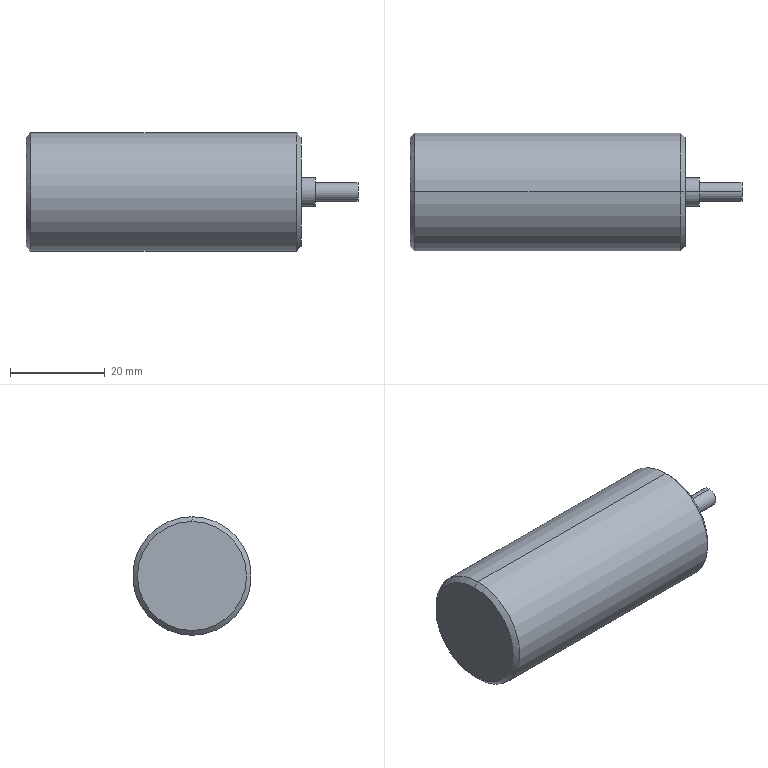Part | SolidWorks | features ICE 3, Chamfer 2, Extrusion 1 | 1 solid | 20 faces | box 70 x 25 x 25 mm | volume 28507 mm3 | cylinder 10 | plane 6 | cone 4 | commonest cylinder face diameters 3 x4 4 x2 6 x2 25 x2
STEP:
#1=CARTESIAN_POINT('',(0.,0.,11.5));
#2=VERTEX_POINT('',#1);
#3=CARTESIAN_POINT('',(0.,0.,-11.5));
#4=VERTEX_POINT('',#3);
#5=CARTESIAN_POINT('',(0.,0.,0.));
#6=DIRECTION('',(-1.,0.,0.));
#7=DIRECTION('',(0.,0.,-1.));
#8=AXIS2_PLACEMENT_3D('',#5,#6,#7);
#9=CIRCLE('',#8,11.5);
#10=EDGE_CURVE('',#2,#4,#9,.T.);
#11=ORIENTED_EDGE('',*,*,#10,.F.);
#12=CARTESIAN_POINT('',(1.,0.,12.5));
#13=VERTEX_POINT('',#12);
#14=CARTESIAN_POINT('',(1.,0.,12.5));
#15=DIRECTION('',(0.7071,0.,0.7071));
#16=VECTOR('',#15,1000.);
#17=LINE('',#14,#16);
#18=EDGE_CURVE('',#2,#13,#17,.T.);
#19=ORIENTED_EDGE('',*,*,#18,.T.);
#20=CARTESIAN_POINT('',(1.,0.,-12.5));
#21=VERTEX_POINT('',#20);
#22=CARTESIAN_POINT('',(1.,0.,0.));
#23=DIRECTION('',(1.,0.,0.));
#24=DIRECTION('',(0.,0.,-1.));
#25=AXIS2_PLACEMENT_3D('',#22,#23,#24);
#26=CIRCLE('',#25,12.5);
#27=EDGE_CURVE('',#21,#13,#26,.T.);
#28=ORIENTED_EDGE('',*,*,#27,.F.);
#29=CARTESIAN_POINT('',(1.,0.,-12.5));
#30=DIRECTION('',(0.7071,0.,-0.7071));
#31=VECTOR('',#30,1000.);
#32=LINE('',#29,#31);
#33=EDGE_CURVE('',#4,#21,#32,.T.);
#34=ORIENTED_EDGE('',*,*,#33,.F.);
#35=EDGE_LOOP('',(#11,#19,#28,#34));
#36=FACE_OUTER_BOUND('',#35,.T.);
#37=CARTESIAN_POINT('',(1.,0.,0.));
#38=DIRECTION('',(1.,0.,0.));
#39=DIRECTION('',(0.,0.,-1.));
#40=AXIS2_PLACEMENT_3D('',#37,#38,#39);
#41=CONICAL_SURFACE('',#40,12.5,0.7854);
#42=ADVANCED_FACE('',(#36),#41,.T.);
#43=CARTESIAN_POINT('',(58.,0.,-11.5));
#44=VERTEX_POINT('',#43);
#45=CARTESIAN_POINT('',(58.,0.,11.5));
#46=VERTEX_POINT('',#45);
#47=CARTESIAN_POINT('',(58.,0.,0.));
#48=DIRECTION('',(1.,0.,0.));
#49=DIRECTION('',(0.,0.,-1.));
#50=AXIS2_PLACEMENT_3D('',#47,#48,#49);
#51=CIRCLE('',#50,11.5);
#52=EDGE_CURVE('',#44,#46,#51,.T.);
#53=ORIENTED_EDGE('',*,*,#52,.F.);
#54=CARTESIAN_POINT('',(57.,0.,-12.5));
#55=VERTEX_POINT('',#54);
#56=CARTESIAN_POINT('',(58.,0.,-11.5));
#57=DIRECTION('',(-0.7071,0.,-0.7071));
#58=VECTOR('',#57,1000.);
#59=LINE('',#56,#58);
#60=EDGE_CURVE('',#44,#55,#59,.T.);
#61=ORIENTED_EDGE('',*,*,#60,.T.);
#62=CARTESIAN_POINT('',(57.,0.,12.5));
#63=VERTEX_POINT('',#62);
#64=CARTESIAN_POINT('',(57.,0.,0.));
#65=DIRECTION('',(-1.,0.,0.));
#66=DIRECTION('',(0.,0.,-1.));
#67=AXIS2_PLACEMENT_3D('',#64,#65,#66);
#68=CIRCLE('',#67,12.5);
#69=EDGE_CURVE('',#63,#55,#68,.T.);
#70=ORIENTED_EDGE('',*,*,#69,.F.);
#71=CARTESIAN_POINT('',(58.,0.,11.5));
#72=DIRECTION('',(-0.7071,0.,0.7071));
#73=VECTOR('',#72,1000.);
#74=LINE('',#71,#73);
#75=EDGE_CURVE('',#46,#63,#74,.T.);
#76=ORIENTED_EDGE('',*,*,#75,.F.);
#77=EDGE_LOOP('',(#53,#61,#70,#76));
#78=FACE_OUTER_BOUND('',#77,.T.);
#79=CARTESIAN_POINT('',(58.,0.,0.));
#80=DIRECTION('',(-1.,0.,0.));
#81=DIRECTION('',(0.,0.,1.));
#82=AXIS2_PLACEMENT_3D('',#79,#80,#81);
#83=CONICAL_SURFACE('',#82,11.5,0.7854);
#84=ADVANCED_FACE('',(#78),#83,.T.);
#85=CARTESIAN_POINT('',(52.,8.5,1.5));
#86=VERTEX_POINT('',#85);
#87=CARTESIAN_POINT('',(52.,8.5,-1.5));
#88=VERTEX_POINT('',#87);
#89=CARTESIAN_POINT('',(52.,8.5,0.));
#90=DIRECTION('',(1.,0.,0.));
#91=DIRECTION('',(0.,0.,-1.));
#92=AXIS2_PLACEMENT_3D('',#89,#90,#91);
#93=CIRCLE('',#92,1.5);
#94=EDGE_CURVE('',#86,#88,#93,.T.);
#95=ORIENTED_EDGE('',*,*,#94,.F.);
#96=CARTESIAN_POINT('',(58.,8.5,1.5));
#97=VERTEX_POINT('',#96);
#98=CARTESIAN_POINT('',(52.,8.5,1.5));
#99=DIRECTION('',(1.,0.,0.));
#100=VECTOR('',#99,1000.);
#101=LINE('',#98,#100);
#102=EDGE_CURVE('',#86,#97,#101,.T.);
#103=ORIENTED_EDGE('',*,*,#102,.T.);
#104=CARTESIAN_POINT('',(58.,8.5,-1.5));
#105=VERTEX_POINT('',#104);
#106=CARTESIAN_POINT('',(58.,8.5,0.));
#107=DIRECTION('',(1.,0.,0.));
#108=DIRECTION('',(0.,0.,-1.));
#109=AXIS2_PLACEMENT_3D('',#106,#107,#108);
#110=CIRCLE('',#109,1.5);
#111=EDGE_CURVE('',#97,#105,#110,.T.);
#112=ORIENTED_EDGE('',*,*,#111,.T.);
#113=CARTESIAN_POINT('',(52.,8.5,-1.5));
#114=DIRECTION('',(1.,0.,0.));
#115=VECTOR('',#114,1000.);
#116=LINE('',#113,#115);
#117=EDGE_CURVE('',#88,#105,#116,.T.);
#118=ORIENTED_EDGE('',*,*,#117,.F.);
#119=EDGE_LOOP('',(#95,#103,#112,#118));
#120=FACE_OUTER_BOUND('',#119,.T.);
#121=CARTESIAN_POINT('',(52.,8.5,0.));
#122=DIRECTION('',(1.,0.,0.));
#123=DIRECTION('',(0.,0.,-1.));
#124=AXIS2_PLACEMENT_3D('',#121,#122,#123);
#125=CYLINDRICAL_SURFACE('',#124,1.5);
#126=ADVANCED_FACE('',(#120),#125,.F.);
#127=CARTESIAN_POINT('',(52.,-8.5,1.5));
#128=VERTEX_POINT('',#127);
#129=CARTESIAN_POINT('',(52.,-8.5,-1.5));
#130=VERTEX_POINT('',#129);
#131=CARTESIAN_POINT('',(52.,-8.5,0.));
#132=DIRECTION('',(1.,0.,0.));
#133=DIRECTION('',(0.,0.,1.));
#134=AXIS2_PLACEMENT_3D('',#131,#132,#133);
#135=CIRCLE('',#134,1.5);
#136=EDGE_CURVE('',#128,#130,#135,.T.);
#137=ORIENTED_EDGE('',*,*,#136,.F.);
#138=CARTESIAN_POINT('',(58.,-8.5,1.5));
#139=VERTEX_POINT('',#138);
#140=CARTESIAN_POINT('',(52.,-8.5,1.5));
#141=DIRECTION('',(1.,0.,0.));
#142=VECTOR('',#141,1000.);
#143=LINE('',#140,#142);
#144=EDGE_CURVE('',#128,#139,#143,.T.);
#145=ORIENTED_EDGE('',*,*,#144,.T.);
#146=CARTESIAN_POINT('',(58.,-8.5,-1.5));
#147=VERTEX_POINT('',#146);
#148=CARTESIAN_POINT('',(58.,-8.5,0.));
#149=DIRECTION('',(1.,0.,0.));
#150=DIRECTION('',(0.,0.,1.));
#151=AXIS2_PLACEMENT_3D('',#148,#149,#150);
#152=CIRCLE('',#151,1.5);
#153=EDGE_CURVE('',#139,#147,#152,.T.);
#154=ORIENTED_EDGE('',*,*,#153,.T.);
#155=CARTESIAN_POINT('',(52.,-8.5,-1.5));
#156=DIRECTION('',(1.,0.,0.));
#157=VECTOR('',#156,1000.);
#158=LINE('',#155,#157);
#159=EDGE_CURVE('',#130,#147,#158,.T.);
#160=ORIENTED_EDGE('',*,*,#159,.F.);
#161=EDGE_LOOP('',(#137,#145,#154,#160));
#162=FACE_OUTER_BOUND('',#161,.T.);
#163=CARTESIAN_POINT('',(52.,-8.5,0.));
#164=DIRECTION('',(1.,0.,0.));
#165=DIRECTION('',(0.,0.,-1.));
#166=AXIS2_PLACEMENT_3D('',#163,#164,#165);
#167=CYLINDRICAL_SURFACE('',#166,1.5);
#168=ADVANCED_FACE('',(#162),#167,.F.);
#169=CARTESIAN_POINT('',(70.,0.,-2.));
#170=VERTEX_POINT('',#169);
#171=CARTESIAN_POINT('',(70.,0.,2.));
#172=VERTEX_POINT('',#171);
#173=CARTESIAN_POINT('',(70.,0.,0.));
#174=DIRECTION('',(1.,0.,0.));
#175=DIRECTION('',(0.,0.,-1.));
#176=AXIS2_PLACEMENT_3D('',#173,#174,#175);
#177=CIRCLE('',#176,2.);
#178=EDGE_CURVE('',#170,#172,#177,.T.);
#179=ORIENTED_EDGE('',*,*,#178,.F.);
#180=CARTESIAN_POINT('',(61.,0.,-2.));
#181=VERTEX_POINT('',#180);
#182=CARTESIAN_POINT('',(70.,0.,-2.));
#183=DIRECTION('',(-1.,0.,0.));
#184=VECTOR('',#183,1000.);
#185=LINE('',#182,#184);
#186=EDGE_CURVE('',#170,#181,#185,.T.);
#187=ORIENTED_EDGE('',*,*,#186,.T.);
#188=CARTESIAN_POINT('',(61.,0.,2.));
#189=VERTEX_POINT('',#188);
#190=CARTESIAN_POINT('',(61.,0.,0.));
#191=DIRECTION('',(1.,0.,0.));
#192=DIRECTION('',(0.,0.,-1.));
#193=AXIS2_PLACEMENT_3D('',#190,#191,#192);
#194=CIRCLE('',#193,2.);
#195=EDGE_CURVE('',#181,#189,#194,.T.);
#196=ORIENTED_EDGE('',*,*,#195,.T.);
#197=CARTESIAN_POINT('',(70.,0.,2.));
#198=DIRECTION('',(-1.,0.,0.));
#199=VECTOR('',#198,1000.);
#200=LINE('',#197,#199);
#201=EDGE_CURVE('',#172,#189,#200,.T.);
#202=ORIENTED_EDGE('',*,*,#201,.F.);
#203=EDGE_LOOP('',(#179,#187,#196,#202));
#204=FACE_OUTER_BOUND('',#203,.T.);
#205=CARTESIAN_POINT('',(70.,0.,0.));
#206=DIRECTION('',(-1.,0.,0.));
#207=DIRECTION('',(0.,0.,1.));
#208=AXIS2_PLACEMENT_3D('',#205,#206,#207);
#209=CYLINDRICAL_SURFACE('',#208,2.);
#210=ADVANCED_FACE('',(#204),#209,.T.);
#211=CARTESIAN_POINT('',(61.,0.,-3.));
#212=VERTEX_POINT('',#211);
#213=CARTESIAN_POINT('',(61.,0.,3.));
#214=VERTEX_POINT('',#213);
#215=CARTESIAN_POINT('',(61.,0.,0.));
#216=DIRECTION('',(1.,0.,0.));
#217=DIRECTION('',(0.,0.,-1.));
#218=AXIS2_PLACEMENT_3D('',#215,#216,#217);
#219=CIRCLE('',#218,3.);
#220=EDGE_CURVE('',#212,#214,#219,.T.);
#221=ORIENTED_EDGE('',*,*,#220,.F.);
#222=CARTESIAN_POINT('',(58.,0.,-3.));
#223=VERTEX_POINT('',#222);
#224=CARTESIAN_POINT('',(61.,0.,-3.));
#225=DIRECTION('',(-1.,0.,0.));
#226=VECTOR('',#225,1000.);
#227=LINE('',#224,#226);
#228=EDGE_CURVE('',#212,#223,#227,.T.);
#229=ORIENTED_EDGE('',*,*,#228,.T.);
#230=CARTESIAN_POINT('',(58.,0.,3.));
#231=VERTEX_POINT('',#230);
#232=CARTESIAN_POINT('',(58.,0.,0.));
#233=DIRECTION('',(1.,0.,0.));
#234=DIRECTION('',(0.,0.,-1.));
#235=AXIS2_PLACEMENT_3D('',#232,#233,#234);
#236=CIRCLE('',#235,3.);
#237=EDGE_CURVE('',#223,#231,#236,.T.);
#238=ORIENTED_EDGE('',*,*,#237,.T.);
#239=CARTESIAN_POINT('',(61.,0.,3.));
#240=DIRECTION('',(-1.,0.,0.));
#241=VECTOR('',#240,1000.);
#242=LINE('',#239,#241);
#243=EDGE_CURVE('',#214,#231,#242,.T.);
#244=ORIENTED_EDGE('',*,*,#243,.F.);
#245=EDGE_LOOP('',(#221,#229,#238,#244));
#246=FACE_OUTER_BOUND('',#245,.T.);
#247=CARTESIAN_POINT('',(61.,0.,0.));
#248=DIRECTION('',(-1.,0.,0.));
#249=DIRECTION('',(0.,0.,1.));
#250=AXIS2_PLACEMENT_3D('',#247,#248,#249);
#251=CYLINDRICAL_SURFACE('',#250,3.);
#252=ADVANCED_FACE('',(#246),#251,.T.);
#253=ORIENTED_EDGE('',*,*,#69,.T.);
#254=CARTESIAN_POINT('',(58.,0.,-12.5));
#255=DIRECTION('',(-1.,0.,0.));
#256=VECTOR('',#255,1000.);
#257=LINE('',#254,#256);
#258=EDGE_CURVE('',#55,#21,#257,.T.);
#259=ORIENTED_EDGE('',*,*,#258,.T.);
#260=ORIENTED_EDGE('',*,*,#27,.T.);
#261=CARTESIAN_POINT('',(58.,0.,12.5));
#262=DIRECTION('',(-1.,0.,0.));
#263=VECTOR('',#262,1000.);
#264=LINE('',#261,#263);
#265=EDGE_CURVE('',#63,#13,#264,.T.);
#266=ORIENTED_EDGE('',*,*,#265,.F.);
#267=EDGE_LOOP('',(#253,#259,#260,#266));
#268=FACE_OUTER_BOUND('',#267,.T.);
#269=CARTESIAN_POINT('',(58.,0.,0.));
#270=DIRECTION('',(-1.,0.,0.));
#271=DIRECTION('',(0.,0.,1.));
#272=AXIS2_PLACEMENT_3D('',#269,#270,#271);
#273=CYLINDRICAL_SURFACE('',#272,12.5);
#274=ADVANCED_FACE('',(#268),#273,.T.);
#275=ORIENTED_EDGE('',*,*,#258,.F.);
#276=CARTESIAN_POINT('',(57.,0.,0.));
#277=DIRECTION('',(-1.,0.,0.));
#278=DIRECTION('',(0.,0.,-1.));
#279=AXIS2_PLACEMENT_3D('',#276,#277,#278);
#280=CIRCLE('',#279,12.5);
#281=EDGE_CURVE('',#55,#63,#280,.T.);
#282=ORIENTED_EDGE('',*,*,#281,.T.);
#283=ORIENTED_EDGE('',*,*,#265,.T.);
#284=CARTESIAN_POINT('',(1.,0.,0.));
#285=DIRECTION('',(1.,0.,0.));
#286=DIRECTION('',(0.,0.,-1.));
#287=AXIS2_PLACEMENT_3D('',#284,#285,#286);
#288=CIRCLE('',#287,12.5);
#289=EDGE_CURVE('',#13,#21,#288,.T.);
#290=ORIENTED_EDGE('',*,*,#289,.T.);
#291=EDGE_LOOP('',(#275,#282,#283,#290));
#292=FACE_OUTER_BOUND('',#291,.T.);
#293=CARTESIAN_POINT('',(58.,0.,0.));
#294=DIRECTION('',(-1.,0.,0.));
#295=DIRECTION('',(0.,0.,1.));
#296=AXIS2_PLACEMENT_3D('',#293,#294,#295);
#297=CYLINDRICAL_SURFACE('',#296,12.5);
#298=ADVANCED_FACE('',(#292),#297,.T.);
#299=CARTESIAN_POINT('',(58.,0.,0.));
#300=DIRECTION('',(1.,0.,0.));
#301=DIRECTION('',(0.,0.,-1.));
#302=AXIS2_PLACEMENT_3D('',#299,#300,#301);
#303=CIRCLE('',#302,11.5);
#304=EDGE_CURVE('',#46,#44,#303,.T.);
#305=ORIENTED_EDGE('',*,*,#304,.T.);
#306=ORIENTED_EDGE('',*,*,#52,.T.);
#307=EDGE_LOOP('',(#305,#306));
#308=FACE_OUTER_BOUND('',#307,.T.);
#309=CARTESIAN_POINT('',(58.,8.5,0.));
#310=DIRECTION('',(1.,0.,0.));
#311=DIRECTION('',(0.,0.,-1.));
#312=AXIS2_PLACEMENT_3D('',#309,#310,#311);
#313=CIRCLE('',#312,1.5);
#314=EDGE_CURVE('',#105,#97,#313,.T.);
#315=ORIENTED_EDGE('',*,*,#314,.F.);
#316=ORIENTED_EDGE('',*,*,#111,.F.);
#317=EDGE_LOOP('',(#315,#316));
#318=FACE_BOUND('',#317,.T.);
#319=CARTESIAN_POINT('',(58.,-8.5,0.));
#320=DIRECTION('',(1.,0.,0.));
#321=DIRECTION('',(0.,0.,1.));
#322=AXIS2_PLACEMENT_3D('',#319,#320,#321);
#323=CIRCLE('',#322,1.5);
#324=EDGE_CURVE('',#147,#139,#323,.T.);
#325=ORIENTED_EDGE('',*,*,#324,.F.);
#326=ORIENTED_EDGE('',*,*,#153,.F.);
#327=EDGE_LOOP('',(#325,#326));
#328=FACE_BOUND('',#327,.T.);
#329=CARTESIAN_POINT('',(58.,0.,0.));
#330=DIRECTION('',(1.,0.,0.));
#331=DIRECTION('',(0.,0.,-1.));
#332=AXIS2_PLACEMENT_3D('',#329,#330,#331);
#333=CIRCLE('',#332,3.);
#334=EDGE_CURVE('',#231,#223,#333,.T.);
#335=ORIENTED_EDGE('',*,*,#334,.F.);
#336=ORIENTED_EDGE('',*,*,#237,.F.);
#337=EDGE_LOOP('',(#335,#336));
#338=FACE_BOUND('',#337,.T.);
#339=CARTESIAN_POINT('',(58.,0.,0.));
#340=DIRECTION('',(1.,0.,0.));
#341=DIRECTION('',(0.,0.,-1.));
#342=AXIS2_PLACEMENT_3D('',#339,#340,#341);
#343=PLANE('',#342);
#344=ADVANCED_FACE('',(#308,#318,#328,#338),#343,.T.);
#345=CARTESIAN_POINT('',(0.,0.,0.));
#346=DIRECTION('',(-1.,0.,0.));
#347=DIRECTION('',(0.,0.,-1.));
#348=AXIS2_PLACEMENT_3D('',#345,#346,#347);
#349=CIRCLE('',#348,11.5);
#350=EDGE_CURVE('',#4,#2,#349,.T.);
#351=ORIENTED_EDGE('',*,*,#350,.T.);
#352=ORIENTED_EDGE('',*,*,#10,.T.);
#353=EDGE_LOOP('',(#351,#352));
#354=FACE_OUTER_BOUND('',#353,.T.);
#355=CARTESIAN_POINT('',(0.,0.,0.));
#356=DIRECTION('',(1.,0.,0.));
#357=DIRECTION('',(0.,0.,-1.));
#358=AXIS2_PLACEMENT_3D('',#355,#356,#357);
#359=PLANE('',#358);
#360=ADVANCED_FACE('',(#354),#359,.F.);
#361=ORIENTED_EDGE('',*,*,#228,.F.);
#362=CARTESIAN_POINT('',(61.,0.,0.));
#363=DIRECTION('',(1.,0.,0.));
#364=DIRECTION('',(0.,0.,-1.));
#365=AXIS2_PLACEMENT_3D('',#362,#363,#364);
#366=CIRCLE('',#365,3.);
#367=EDGE_CURVE('',#214,#212,#366,.T.);
#368=ORIENTED_EDGE('',*,*,#367,.F.);
#369=ORIENTED_EDGE('',*,*,#243,.T.);
#370=ORIENTED_EDGE('',*,*,#334,.T.);
#371=EDGE_LOOP('',(#361,#368,#369,#370));
#372=FACE_OUTER_BOUND('',#371,.T.);
#373=CARTESIAN_POINT('',(61.,0.,0.));
#374=DIRECTION('',(-1.,0.,0.));
#375=DIRECTION('',(0.,0.,1.));
#376=AXIS2_PLACEMENT_3D('',#373,#374,#375);
#377=CYLINDRICAL_SURFACE('',#376,3.);
#378=ADVANCED_FACE('',(#372),#377,.T.);
#379=CARTESIAN_POINT('',(61.,0.,0.));
#380=DIRECTION('',(1.,0.,0.));
#381=DIRECTION('',(0.,0.,-1.));
#382=AXIS2_PLACEMENT_3D('',#379,#380,#381);
#383=CIRCLE('',#382,2.);
#384=EDGE_CURVE('',#189,#181,#383,.T.);
#385=ORIENTED_EDGE('',*,*,#384,.F.);
#386=ORIENTED_EDGE('',*,*,#195,.F.);
#387=EDGE_LOOP('',(#385,#386));
#388=FACE_BOUND('',#387,.T.);
#389=ORIENTED_EDGE('',*,*,#367,.T.);
#390=ORIENTED_EDGE('',*,*,#220,.T.);
#391=EDGE_LOOP('',(#389,#390));
#392=FACE_OUTER_BOUND('',#391,.T.);
#393=CARTESIAN_POINT('',(61.,0.,0.));
#394=DIRECTION('',(1.,0.,0.));
#395=DIRECTION('',(0.,0.,-1.));
#396=AXIS2_PLACEMENT_3D('',#393,#394,#395);
#397=PLANE('',#396);
#398=ADVANCED_FACE('',(#388,#392),#397,.T.);
#399=ORIENTED_EDGE('',*,*,#186,.F.);
#400=CARTESIAN_POINT('',(70.,0.,0.));
#401=DIRECTION('',(1.,0.,0.));
#402=DIRECTION('',(0.,0.,-1.));
#403=AXIS2_PLACEMENT_3D('',#400,#401,#402);
#404=CIRCLE('',#403,2.);
#405=EDGE_CURVE('',#172,#170,#404,.T.);
#406=ORIENTED_EDGE('',*,*,#405,.F.);
#407=ORIENTED_EDGE('',*,*,#201,.T.);
#408=ORIENTED_EDGE('',*,*,#384,.T.);
#409=EDGE_LOOP('',(#399,#406,#407,#408));
#410=FACE_OUTER_BOUND('',#409,.T.);
#411=CARTESIAN_POINT('',(70.,0.,0.));
#412=DIRECTION('',(-1.,0.,0.));
#413=DIRECTION('',(0.,0.,1.));
#414=AXIS2_PLACEMENT_3D('',#411,#412,#413);
#415=CYLINDRICAL_SURFACE('',#414,2.);
#416=ADVANCED_FACE('',(#410),#415,.T.);
#417=ORIENTED_EDGE('',*,*,#405,.T.);
#418=ORIENTED_EDGE('',*,*,#178,.T.);
#419=EDGE_LOOP('',(#417,#418));
#420=FACE_OUTER_BOUND('',#419,.T.);
#421=CARTESIAN_POINT('',(70.,0.,0.));
#422=DIRECTION('',(1.,0.,0.));
#423=DIRECTION('',(0.,0.,-1.));
#424=AXIS2_PLACEMENT_3D('',#421,#422,#423);
#425=PLANE('',#424);
#426=ADVANCED_FACE('',(#420),#425,.T.);
#427=ORIENTED_EDGE('',*,*,#144,.F.);
#428=CARTESIAN_POINT('',(52.,-8.5,0.));
#429=DIRECTION('',(1.,0.,0.));
#430=DIRECTION('',(0.,0.,1.));
#431=AXIS2_PLACEMENT_3D('',#428,#429,#430);
#432=CIRCLE('',#431,1.5);
#433=EDGE_CURVE('',#130,#128,#432,.T.);
#434=ORIENTED_EDGE('',*,*,#433,.F.);
#435=ORIENTED_EDGE('',*,*,#159,.T.);
#436=ORIENTED_EDGE('',*,*,#324,.T.);
#437=EDGE_LOOP('',(#427,#434,#435,#436));
#438=FACE_OUTER_BOUND('',#437,.T.);
#439=CARTESIAN_POINT('',(52.,-8.5,0.));
#440=DIRECTION('',(1.,0.,0.));
#441=DIRECTION('',(0.,0.,-1.));
#442=AXIS2_PLACEMENT_3D('',#439,#440,#441);
#443=CYLINDRICAL_SURFACE('',#442,1.5);
#444=ADVANCED_FACE('',(#438),#443,.F.);
#445=ORIENTED_EDGE('',*,*,#433,.T.);
#446=ORIENTED_EDGE('',*,*,#136,.T.);
#447=EDGE_LOOP('',(#445,#446));
#448=FACE_OUTER_BOUND('',#447,.T.);
#449=CARTESIAN_POINT('',(52.,-8.5,0.));
#450=DIRECTION('',(-1.,0.,0.));
#451=DIRECTION('',(0.,0.,1.));
#452=AXIS2_PLACEMENT_3D('',#449,#450,#451);
#453=PLANE('',#452);
#454=ADVANCED_FACE('',(#448),#453,.F.);
#455=ORIENTED_EDGE('',*,*,#102,.F.);
#456=CARTESIAN_POINT('',(52.,8.5,0.));
#457=DIRECTION('',(1.,0.,0.));
#458=DIRECTION('',(0.,0.,-1.));
#459=AXIS2_PLACEMENT_3D('',#456,#457,#458);
#460=CIRCLE('',#459,1.5);
#461=EDGE_CURVE('',#88,#86,#460,.T.);
#462=ORIENTED_EDGE('',*,*,#461,.F.);
#463=ORIENTED_EDGE('',*,*,#117,.T.);
#464=ORIENTED_EDGE('',*,*,#314,.T.);
#465=EDGE_LOOP('',(#455,#462,#463,#464));
#466=FACE_OUTER_BOUND('',#465,.T.);
#467=CARTESIAN_POINT('',(52.,8.5,0.));
#468=DIRECTION('',(1.,0.,0.));
#469=DIRECTION('',(0.,0.,-1.));
#470=AXIS2_PLACEMENT_3D('',#467,#468,#469);
#471=CYLINDRICAL_SURFACE('',#470,1.5);
#472=ADVANCED_FACE('',(#466),#471,.F.);
#473=ORIENTED_EDGE('',*,*,#461,.T.);
#474=ORIENTED_EDGE('',*,*,#94,.T.);
#475=EDGE_LOOP('',(#473,#474));
#476=FACE_OUTER_BOUND('',#475,.T.);
#477=CARTESIAN_POINT('',(52.,8.5,0.));
#478=DIRECTION('',(1.,0.,0.));
#479=DIRECTION('',(0.,0.,-1.));
#480=AXIS2_PLACEMENT_3D('',#477,#478,#479);
#481=PLANE('',#480);
#482=ADVANCED_FACE('',(#476),#481,.T.);
#483=ORIENTED_EDGE('',*,*,#60,.F.);
#484=ORIENTED_EDGE('',*,*,#304,.F.);
#485=ORIENTED_EDGE('',*,*,#75,.T.);
#486=ORIENTED_EDGE('',*,*,#281,.F.);
#487=EDGE_LOOP('',(#483,#484,#485,#486));
#488=FACE_OUTER_BOUND('',#487,.T.);
#489=CARTESIAN_POINT('',(58.,0.,0.));
#490=DIRECTION('',(-1.,0.,0.));
#491=DIRECTION('',(0.,0.,1.));
#492=AXIS2_PLACEMENT_3D('',#489,#490,#491);
#493=CONICAL_SURFACE('',#492,11.5,0.7854);
#494=ADVANCED_FACE('',(#488),#493,.T.);
#495=ORIENTED_EDGE('',*,*,#18,.F.);
#496=ORIENTED_EDGE('',*,*,#350,.F.);
#497=ORIENTED_EDGE('',*,*,#33,.T.);
#498=ORIENTED_EDGE('',*,*,#289,.F.);
#499=EDGE_LOOP('',(#495,#496,#497,#498));
#500=FACE_OUTER_BOUND('',#499,.T.);
#501=CARTESIAN_POINT('',(1.,0.,0.));
#502=DIRECTION('',(1.,0.,0.));
#503=DIRECTION('',(0.,0.,-1.));
#504=AXIS2_PLACEMENT_3D('',#501,#502,#503);
#505=CONICAL_SURFACE('',#504,12.5,0.7854);
#506=ADVANCED_FACE('',(#500),#505,.T.);
#507=CLOSED_SHELL('',(#42,#84,#126,#168,#210,#252,#274,#298,#344,#360,#378,#398,#416,#426,#444,#454,#472,#482,#494,#506));
#508=MANIFOLD_SOLID_BREP('',#507);
#509=CARTESIAN_POINT('',(0.,0.,0.));
#510=DIRECTION('',(0.,0.,1.));
#511=DIRECTION('',(1.,0.,0.));
#512=AXIS2_PLACEMENT_3D('',#509,#510,#511);
#513=(LENGTH_UNIT()NAMED_UNIT(*)SI_UNIT(.MILLI.,.METRE.));
#514=UNCERTAINTY_MEASURE_WITH_UNIT(LENGTH_MEASURE(0.00001),#513,'','');
#515=(NAMED_UNIT(*)PLANE_ANGLE_UNIT()SI_UNIT($,.RADIAN.));
#516=(NAMED_UNIT(*)SI_UNIT($,.STERADIAN.)SOLID_ANGLE_UNIT());
#517=(GEOMETRIC_REPRESENTATION_CONTEXT(3)GLOBAL_UNCERTAINTY_ASSIGNED_CONTEXT((#514))GLOBAL_UNIT_ASSIGNED_CONTEXT((#513,#515,#516))REPRESENTATION_CONTEXT('',''));
#518=ADVANCED_BREP_SHAPE_REPRESENTATION('',(#508,#512),#517);